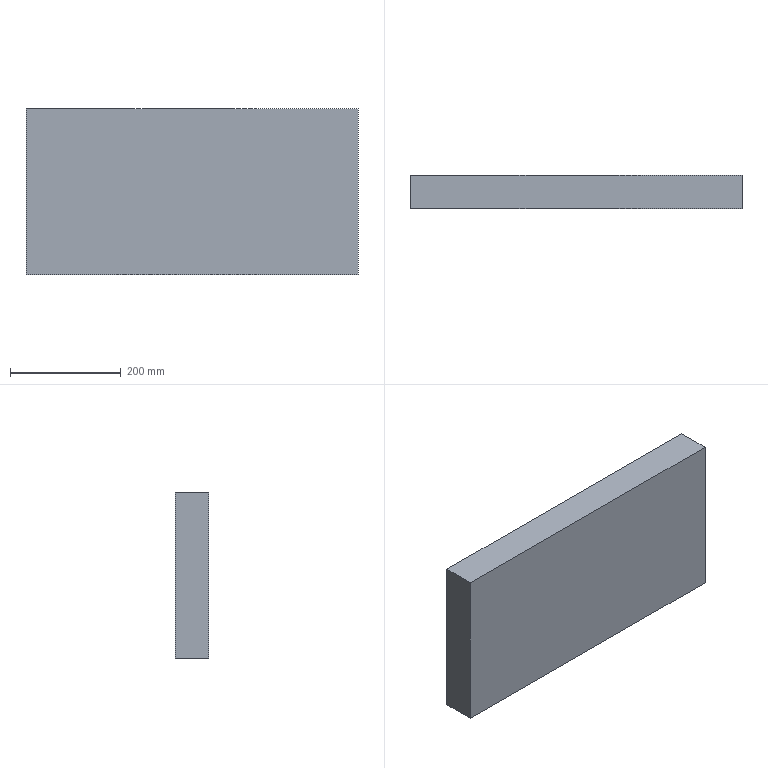Part | SolidWorks | features Cut 3, Extrusion 1, LPattern 1 | 1 solid | 76 faces | box 600 x 60 x 300 mm | volume 7453417 mm3 | plane 56 | cylinder 20 | commonest cylinder face diameters 85 x20